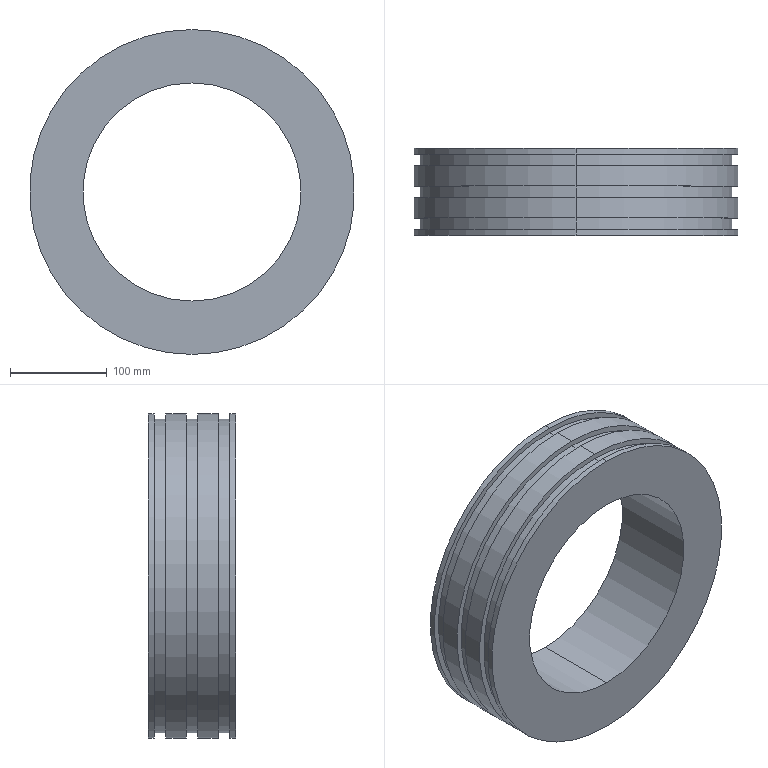Part | SolidWorks | features BaseBody 1, Scale 1 | 1 solid | 24 faces | box 336 x 90 x 336 mm | volume 4158634 mm3 | cylinder 16 | plane 8 | commonest cylinder face diameters 336 x8 324 x6 225.6 x2
STEP:
#1=CARTESIAN_POINT('',(0.,82.5,112.8));
#2=VERTEX_POINT('',#1);
#3=CARTESIAN_POINT('',(0.,82.5,-112.8));
#4=VERTEX_POINT('',#3);
#5=CARTESIAN_POINT('',(0.,82.5,0.));
#6=DIRECTION('',(0.,-1.,0.));
#7=DIRECTION('',(0.,0.,-1.));
#8=AXIS2_PLACEMENT_3D('',#5,#6,#7);
#9=CIRCLE('',#8,112.8);
#10=EDGE_CURVE('',#2,#4,#9,.T.);
#11=ORIENTED_EDGE('',*,*,#10,.F.);
#12=CARTESIAN_POINT('',(0.,-7.5,112.8));
#13=VERTEX_POINT('',#12);
#14=CARTESIAN_POINT('',(0.,82.5,112.8));
#15=DIRECTION('',(0.,-1.,0.));
#16=VECTOR('',#15,1000.);
#17=LINE('',#14,#16);
#18=EDGE_CURVE('',#2,#13,#17,.T.);
#19=ORIENTED_EDGE('',*,*,#18,.T.);
#20=CARTESIAN_POINT('',(0.,-7.5,-112.8));
#21=VERTEX_POINT('',#20);
#22=CARTESIAN_POINT('',(0.,-7.5,0.));
#23=DIRECTION('',(0.,1.,0.));
#24=DIRECTION('',(0.,0.,-1.));
#25=AXIS2_PLACEMENT_3D('',#22,#23,#24);
#26=CIRCLE('',#25,112.8);
#27=EDGE_CURVE('',#21,#13,#26,.T.);
#28=ORIENTED_EDGE('',*,*,#27,.F.);
#29=CARTESIAN_POINT('',(0.,82.5,-112.8));
#30=DIRECTION('',(0.,-1.,0.));
#31=VECTOR('',#30,1000.);
#32=LINE('',#29,#31);
#33=EDGE_CURVE('',#4,#21,#32,.T.);
#34=ORIENTED_EDGE('',*,*,#33,.F.);
#35=EDGE_LOOP('',(#11,#19,#28,#34));
#36=FACE_OUTER_BOUND('',#35,.T.);
#37=CARTESIAN_POINT('',(0.,82.5,0.));
#38=DIRECTION('',(0.,-1.,0.));
#39=DIRECTION('',(0.,0.,-1.));
#40=AXIS2_PLACEMENT_3D('',#37,#38,#39);
#41=CYLINDRICAL_SURFACE('',#40,112.8);
#42=ADVANCED_FACE('',(#36),#41,.F.);
#43=CARTESIAN_POINT('',(0.,82.5,168.));
#44=VERTEX_POINT('',#43);
#45=CARTESIAN_POINT('',(0.,82.5,-168.));
#46=VERTEX_POINT('',#45);
#47=CARTESIAN_POINT('',(0.,82.5,0.));
#48=DIRECTION('',(0.,1.,0.));
#49=DIRECTION('',(0.,0.,-1.));
#50=AXIS2_PLACEMENT_3D('',#47,#48,#49);
#51=CIRCLE('',#50,168.);
#52=EDGE_CURVE('',#44,#46,#51,.T.);
#53=ORIENTED_EDGE('',*,*,#52,.F.);
#54=CARTESIAN_POINT('',(0.,76.5,168.));
#55=VERTEX_POINT('',#54);
#56=CARTESIAN_POINT('',(0.,82.5,168.));
#57=DIRECTION('',(0.,-1.,0.));
#58=VECTOR('',#57,1000.);
#59=LINE('',#56,#58);
#60=EDGE_CURVE('',#44,#55,#59,.T.);
#61=ORIENTED_EDGE('',*,*,#60,.T.);
#62=CARTESIAN_POINT('',(0.,76.5,-168.));
#63=VERTEX_POINT('',#62);
#64=CARTESIAN_POINT('',(0.,76.5,0.));
#65=DIRECTION('',(0.,1.,0.));
#66=DIRECTION('',(0.,0.,-1.));
#67=AXIS2_PLACEMENT_3D('',#64,#65,#66);
#68=CIRCLE('',#67,168.);
#69=EDGE_CURVE('',#55,#63,#68,.T.);
#70=ORIENTED_EDGE('',*,*,#69,.T.);
#71=CARTESIAN_POINT('',(0.,82.5,-168.));
#72=DIRECTION('',(0.,-1.,0.));
#73=VECTOR('',#72,1000.);
#74=LINE('',#71,#73);
#75=EDGE_CURVE('',#46,#63,#74,.T.);
#76=ORIENTED_EDGE('',*,*,#75,.F.);
#77=EDGE_LOOP('',(#53,#61,#70,#76));
#78=FACE_OUTER_BOUND('',#77,.T.);
#79=CARTESIAN_POINT('',(0.,82.5,0.));
#80=DIRECTION('',(0.,-1.,0.));
#81=DIRECTION('',(0.,0.,-1.));
#82=AXIS2_PLACEMENT_3D('',#79,#80,#81);
#83=CYLINDRICAL_SURFACE('',#82,168.);
#84=ADVANCED_FACE('',(#78),#83,.T.);
#85=CARTESIAN_POINT('',(0.,-1.5,-168.));
#86=VERTEX_POINT('',#85);
#87=CARTESIAN_POINT('',(0.,-1.5,168.));
#88=VERTEX_POINT('',#87);
#89=CARTESIAN_POINT('',(0.,-1.5,0.));
#90=DIRECTION('',(0.,-1.,0.));
#91=DIRECTION('',(0.,0.,-1.));
#92=AXIS2_PLACEMENT_3D('',#89,#90,#91);
#93=CIRCLE('',#92,168.);
#94=EDGE_CURVE('',#86,#88,#93,.T.);
#95=ORIENTED_EDGE('',*,*,#94,.T.);
#96=CARTESIAN_POINT('',(0.,-7.5,168.));
#97=VERTEX_POINT('',#96);
#98=CARTESIAN_POINT('',(0.,82.5,168.));
#99=DIRECTION('',(0.,-1.,0.));
#100=VECTOR('',#99,1000.);
#101=LINE('',#98,#100);
#102=EDGE_CURVE('',#88,#97,#101,.T.);
#103=ORIENTED_EDGE('',*,*,#102,.T.);
#104=CARTESIAN_POINT('',(0.,-7.5,-168.));
#105=VERTEX_POINT('',#104);
#106=CARTESIAN_POINT('',(0.,-7.5,0.));
#107=DIRECTION('',(0.,1.,0.));
#108=DIRECTION('',(0.,0.,-1.));
#109=AXIS2_PLACEMENT_3D('',#106,#107,#108);
#110=CIRCLE('',#109,168.);
#111=EDGE_CURVE('',#97,#105,#110,.T.);
#112=ORIENTED_EDGE('',*,*,#111,.T.);
#113=CARTESIAN_POINT('',(0.,82.5,-168.));
#114=DIRECTION('',(0.,-1.,0.));
#115=VECTOR('',#114,1000.);
#116=LINE('',#113,#115);
#117=EDGE_CURVE('',#86,#105,#116,.T.);
#118=ORIENTED_EDGE('',*,*,#117,.F.);
#119=EDGE_LOOP('',(#95,#103,#112,#118));
#120=FACE_OUTER_BOUND('',#119,.T.);
#121=CARTESIAN_POINT('',(0.,82.5,0.));
#122=DIRECTION('',(0.,-1.,0.));
#123=DIRECTION('',(0.,0.,-1.));
#124=AXIS2_PLACEMENT_3D('',#121,#122,#123);
#125=CYLINDRICAL_SURFACE('',#124,168.);
#126=ADVANCED_FACE('',(#120),#125,.T.);
#127=CARTESIAN_POINT('',(0.,76.5,-162.));
#128=VERTEX_POINT('',#127);
#129=CARTESIAN_POINT('',(0.,76.5,162.));
#130=VERTEX_POINT('',#129);
#131=CARTESIAN_POINT('',(0.,76.5,0.));
#132=DIRECTION('',(0.,-1.,0.));
#133=DIRECTION('',(0.,0.,-1.));
#134=AXIS2_PLACEMENT_3D('',#131,#132,#133);
#135=CIRCLE('',#134,162.);
#136=EDGE_CURVE('',#128,#130,#135,.T.);
#137=ORIENTED_EDGE('',*,*,#136,.T.);
#138=CARTESIAN_POINT('',(0.,64.5,162.));
#139=VERTEX_POINT('',#138);
#140=CARTESIAN_POINT('',(0.,-7.5,162.));
#141=DIRECTION('',(0.,-1.,0.));
#142=VECTOR('',#141,1000.);
#143=LINE('',#140,#142);
#144=EDGE_CURVE('',#130,#139,#143,.T.);
#145=ORIENTED_EDGE('',*,*,#144,.T.);
#146=CARTESIAN_POINT('',(0.,64.5,-162.));
#147=VERTEX_POINT('',#146);
#148=CARTESIAN_POINT('',(0.,64.5,0.));
#149=DIRECTION('',(0.,1.,0.));
#150=DIRECTION('',(0.,0.,-1.));
#151=AXIS2_PLACEMENT_3D('',#148,#149,#150);
#152=CIRCLE('',#151,162.);
#153=EDGE_CURVE('',#139,#147,#152,.T.);
#154=ORIENTED_EDGE('',*,*,#153,.T.);
#155=CARTESIAN_POINT('',(0.,-7.5,-162.));
#156=DIRECTION('',(0.,-1.,0.));
#157=VECTOR('',#156,1000.);
#158=LINE('',#155,#157);
#159=EDGE_CURVE('',#128,#147,#158,.T.);
#160=ORIENTED_EDGE('',*,*,#159,.F.);
#161=EDGE_LOOP('',(#137,#145,#154,#160));
#162=FACE_OUTER_BOUND('',#161,.T.);
#163=CARTESIAN_POINT('',(0.,-7.5,0.));
#164=DIRECTION('',(0.,-1.,0.));
#165=DIRECTION('',(0.,0.,-1.));
#166=AXIS2_PLACEMENT_3D('',#163,#164,#165);
#167=CYLINDRICAL_SURFACE('',#166,162.);
#168=ADVANCED_FACE('',(#162),#167,.T.);
#169=CARTESIAN_POINT('',(0.,10.5,-162.));
#170=VERTEX_POINT('',#169);
#171=CARTESIAN_POINT('',(0.,10.5,162.));
#172=VERTEX_POINT('',#171);
#173=CARTESIAN_POINT('',(0.,10.5,0.));
#174=DIRECTION('',(0.,-1.,0.));
#175=DIRECTION('',(0.,0.,-1.));
#176=AXIS2_PLACEMENT_3D('',#173,#174,#175);
#177=CIRCLE('',#176,162.);
#178=EDGE_CURVE('',#170,#172,#177,.T.);
#179=ORIENTED_EDGE('',*,*,#178,.T.);
#180=CARTESIAN_POINT('',(0.,-1.5,162.));
#181=VERTEX_POINT('',#180);
#182=CARTESIAN_POINT('',(0.,-7.5,162.));
#183=DIRECTION('',(0.,-1.,0.));
#184=VECTOR('',#183,1000.);
#185=LINE('',#182,#184);
#186=EDGE_CURVE('',#172,#181,#185,.T.);
#187=ORIENTED_EDGE('',*,*,#186,.T.);
#188=CARTESIAN_POINT('',(0.,-1.5,-162.));
#189=VERTEX_POINT('',#188);
#190=CARTESIAN_POINT('',(0.,-1.5,0.));
#191=DIRECTION('',(0.,1.,0.));
#192=DIRECTION('',(0.,0.,-1.));
#193=AXIS2_PLACEMENT_3D('',#190,#191,#192);
#194=CIRCLE('',#193,162.);
#195=EDGE_CURVE('',#181,#189,#194,.T.);
#196=ORIENTED_EDGE('',*,*,#195,.T.);
#197=CARTESIAN_POINT('',(0.,-7.5,-162.));
#198=DIRECTION('',(0.,-1.,0.));
#199=VECTOR('',#198,1000.);
#200=LINE('',#197,#199);
#201=EDGE_CURVE('',#170,#189,#200,.T.);
#202=ORIENTED_EDGE('',*,*,#201,.F.);
#203=EDGE_LOOP('',(#179,#187,#196,#202));
#204=FACE_OUTER_BOUND('',#203,.T.);
#205=CARTESIAN_POINT('',(0.,-7.5,0.));
#206=DIRECTION('',(0.,-1.,0.));
#207=DIRECTION('',(0.,0.,-1.));
#208=AXIS2_PLACEMENT_3D('',#205,#206,#207);
#209=CYLINDRICAL_SURFACE('',#208,162.);
#210=ADVANCED_FACE('',(#204),#209,.T.);
#211=CARTESIAN_POINT('',(0.,64.5,-168.));
#212=VERTEX_POINT('',#211);
#213=CARTESIAN_POINT('',(0.,64.5,168.));
#214=VERTEX_POINT('',#213);
#215=CARTESIAN_POINT('',(0.,64.5,0.));
#216=DIRECTION('',(0.,-1.,0.));
#217=DIRECTION('',(0.,0.,-1.));
#218=AXIS2_PLACEMENT_3D('',#215,#216,#217);
#219=CIRCLE('',#218,168.);
#220=EDGE_CURVE('',#212,#214,#219,.T.);
#221=ORIENTED_EDGE('',*,*,#220,.T.);
#222=CARTESIAN_POINT('',(0.,43.5,168.));
#223=VERTEX_POINT('',#222);
#224=CARTESIAN_POINT('',(0.,82.5,168.));
#225=DIRECTION('',(0.,-1.,0.));
#226=VECTOR('',#225,1000.);
#227=LINE('',#224,#226);
#228=EDGE_CURVE('',#214,#223,#227,.T.);
#229=ORIENTED_EDGE('',*,*,#228,.T.);
#230=CARTESIAN_POINT('',(0.,43.5,-168.));
#231=VERTEX_POINT('',#230);
#232=CARTESIAN_POINT('',(0.,43.5,0.));
#233=DIRECTION('',(0.,1.,0.));
#234=DIRECTION('',(0.,0.,-1.));
#235=AXIS2_PLACEMENT_3D('',#232,#233,#234);
#236=CIRCLE('',#235,168.);
#237=EDGE_CURVE('',#223,#231,#236,.T.);
#238=ORIENTED_EDGE('',*,*,#237,.T.);
#239=CARTESIAN_POINT('',(0.,82.5,-168.));
#240=DIRECTION('',(0.,-1.,0.));
#241=VECTOR('',#240,1000.);
#242=LINE('',#239,#241);
#243=EDGE_CURVE('',#212,#231,#242,.T.);
#244=ORIENTED_EDGE('',*,*,#243,.F.);
#245=EDGE_LOOP('',(#221,#229,#238,#244));
#246=FACE_OUTER_BOUND('',#245,.T.);
#247=CARTESIAN_POINT('',(0.,82.5,0.));
#248=DIRECTION('',(0.,-1.,0.));
#249=DIRECTION('',(0.,0.,-1.));
#250=AXIS2_PLACEMENT_3D('',#247,#248,#249);
#251=CYLINDRICAL_SURFACE('',#250,168.);
#252=ADVANCED_FACE('',(#246),#251,.T.);
#253=CARTESIAN_POINT('',(0.,31.5,-168.));
#254=VERTEX_POINT('',#253);
#255=CARTESIAN_POINT('',(0.,31.5,168.));
#256=VERTEX_POINT('',#255);
#257=CARTESIAN_POINT('',(0.,31.5,0.));
#258=DIRECTION('',(0.,-1.,0.));
#259=DIRECTION('',(0.,0.,-1.));
#260=AXIS2_PLACEMENT_3D('',#257,#258,#259);
#261=CIRCLE('',#260,168.);
#262=EDGE_CURVE('',#254,#256,#261,.T.);
#263=ORIENTED_EDGE('',*,*,#262,.T.);
#264=CARTESIAN_POINT('',(0.,10.5,168.));
#265=VERTEX_POINT('',#264);
#266=CARTESIAN_POINT('',(0.,82.5,168.));
#267=DIRECTION('',(0.,-1.,0.));
#268=VECTOR('',#267,1000.);
#269=LINE('',#266,#268);
#270=EDGE_CURVE('',#256,#265,#269,.T.);
#271=ORIENTED_EDGE('',*,*,#270,.T.);
#272=CARTESIAN_POINT('',(0.,10.5,-168.));
#273=VERTEX_POINT('',#272);
#274=CARTESIAN_POINT('',(0.,10.5,0.));
#275=DIRECTION('',(0.,1.,0.));
#276=DIRECTION('',(0.,0.,-1.));
#277=AXIS2_PLACEMENT_3D('',#274,#275,#276);
#278=CIRCLE('',#277,168.);
#279=EDGE_CURVE('',#265,#273,#278,.T.);
#280=ORIENTED_EDGE('',*,*,#279,.T.);
#281=CARTESIAN_POINT('',(0.,82.5,-168.));
#282=DIRECTION('',(0.,-1.,0.));
#283=VECTOR('',#282,1000.);
#284=LINE('',#281,#283);
#285=EDGE_CURVE('',#254,#273,#284,.T.);
#286=ORIENTED_EDGE('',*,*,#285,.F.);
#287=EDGE_LOOP('',(#263,#271,#280,#286));
#288=FACE_OUTER_BOUND('',#287,.T.);
#289=CARTESIAN_POINT('',(0.,82.5,0.));
#290=DIRECTION('',(0.,-1.,0.));
#291=DIRECTION('',(0.,0.,-1.));
#292=AXIS2_PLACEMENT_3D('',#289,#290,#291);
#293=CYLINDRICAL_SURFACE('',#292,168.);
#294=ADVANCED_FACE('',(#288),#293,.T.);
#295=CARTESIAN_POINT('',(0.,43.5,-162.));
#296=VERTEX_POINT('',#295);
#297=CARTESIAN_POINT('',(0.,43.5,162.));
#298=VERTEX_POINT('',#297);
#299=CARTESIAN_POINT('',(0.,43.5,0.));
#300=DIRECTION('',(0.,-1.,0.));
#301=DIRECTION('',(0.,0.,-1.));
#302=AXIS2_PLACEMENT_3D('',#299,#300,#301);
#303=CIRCLE('',#302,162.);
#304=EDGE_CURVE('',#296,#298,#303,.T.);
#305=ORIENTED_EDGE('',*,*,#304,.T.);
#306=CARTESIAN_POINT('',(0.,31.5,162.));
#307=VERTEX_POINT('',#306);
#308=CARTESIAN_POINT('',(0.,-7.5,162.));
#309=DIRECTION('',(0.,-1.,0.));
#310=VECTOR('',#309,1000.);
#311=LINE('',#308,#310);
#312=EDGE_CURVE('',#298,#307,#311,.T.);
#313=ORIENTED_EDGE('',*,*,#312,.T.);
#314=CARTESIAN_POINT('',(0.,31.5,-162.));
#315=VERTEX_POINT('',#314);
#316=CARTESIAN_POINT('',(0.,31.5,0.));
#317=DIRECTION('',(0.,1.,0.));
#318=DIRECTION('',(0.,0.,-1.));
#319=AXIS2_PLACEMENT_3D('',#316,#317,#318);
#320=CIRCLE('',#319,162.);
#321=EDGE_CURVE('',#307,#315,#320,.T.);
#322=ORIENTED_EDGE('',*,*,#321,.T.);
#323=CARTESIAN_POINT('',(0.,-7.5,-162.));
#324=DIRECTION('',(0.,-1.,0.));
#325=VECTOR('',#324,1000.);
#326=LINE('',#323,#325);
#327=EDGE_CURVE('',#296,#315,#326,.T.);
#328=ORIENTED_EDGE('',*,*,#327,.F.);
#329=EDGE_LOOP('',(#305,#313,#322,#328));
#330=FACE_OUTER_BOUND('',#329,.T.);
#331=CARTESIAN_POINT('',(0.,-7.5,0.));
#332=DIRECTION('',(0.,-1.,0.));
#333=DIRECTION('',(0.,0.,-1.));
#334=AXIS2_PLACEMENT_3D('',#331,#332,#333);
#335=CYLINDRICAL_SURFACE('',#334,162.);
#336=ADVANCED_FACE('',(#330),#335,.T.);
#337=CARTESIAN_POINT('',(0.,82.5,0.));
#338=DIRECTION('',(0.,-1.,0.));
#339=DIRECTION('',(0.,0.,-1.));
#340=AXIS2_PLACEMENT_3D('',#337,#338,#339);
#341=CIRCLE('',#340,112.8);
#342=EDGE_CURVE('',#4,#2,#341,.T.);
#343=ORIENTED_EDGE('',*,*,#342,.T.);
#344=ORIENTED_EDGE('',*,*,#10,.T.);
#345=EDGE_LOOP('',(#343,#344));
#346=FACE_BOUND('',#345,.T.);
#347=CARTESIAN_POINT('',(0.,82.5,0.));
#348=DIRECTION('',(0.,1.,0.));
#349=DIRECTION('',(0.,0.,-1.));
#350=AXIS2_PLACEMENT_3D('',#347,#348,#349);
#351=CIRCLE('',#350,168.);
#352=EDGE_CURVE('',#46,#44,#351,.T.);
#353=ORIENTED_EDGE('',*,*,#352,.T.);
#354=ORIENTED_EDGE('',*,*,#52,.T.);
#355=EDGE_LOOP('',(#353,#354));
#356=FACE_OUTER_BOUND('',#355,.T.);
#357=CARTESIAN_POINT('',(0.,82.5,0.));
#358=DIRECTION('',(0.,1.,0.));
#359=DIRECTION('',(0.,0.,1.));
#360=AXIS2_PLACEMENT_3D('',#357,#358,#359);
#361=PLANE('',#360);
#362=ADVANCED_FACE('',(#346,#356),#361,.T.);
#363=ORIENTED_EDGE('',*,*,#18,.F.);
#364=ORIENTED_EDGE('',*,*,#342,.F.);
#365=ORIENTED_EDGE('',*,*,#33,.T.);
#366=CARTESIAN_POINT('',(0.,-7.5,0.));
#367=DIRECTION('',(0.,1.,0.));
#368=DIRECTION('',(0.,0.,-1.));
#369=AXIS2_PLACEMENT_3D('',#366,#367,#368);
#370=CIRCLE('',#369,112.8);
#371=EDGE_CURVE('',#13,#21,#370,.T.);
#372=ORIENTED_EDGE('',*,*,#371,.F.);
#373=EDGE_LOOP('',(#363,#364,#365,#372));
#374=FACE_OUTER_BOUND('',#373,.T.);
#375=CARTESIAN_POINT('',(0.,82.5,0.));
#376=DIRECTION('',(0.,-1.,0.));
#377=DIRECTION('',(0.,0.,-1.));
#378=AXIS2_PLACEMENT_3D('',#375,#376,#377);
#379=CYLINDRICAL_SURFACE('',#378,112.8);
#380=ADVANCED_FACE('',(#374),#379,.F.);
#381=ORIENTED_EDGE('',*,*,#60,.F.);
#382=ORIENTED_EDGE('',*,*,#352,.F.);
#383=ORIENTED_EDGE('',*,*,#75,.T.);
#384=CARTESIAN_POINT('',(0.,76.5,0.));
#385=DIRECTION('',(0.,1.,0.));
#386=DIRECTION('',(0.,0.,-1.));
#387=AXIS2_PLACEMENT_3D('',#384,#385,#386);
#388=CIRCLE('',#387,168.);
#389=EDGE_CURVE('',#63,#55,#388,.T.);
#390=ORIENTED_EDGE('',*,*,#389,.T.);
#391=EDGE_LOOP('',(#381,#382,#383,#390));
#392=FACE_OUTER_BOUND('',#391,.T.);
#393=CARTESIAN_POINT('',(0.,82.5,0.));
#394=DIRECTION('',(0.,-1.,0.));
#395=DIRECTION('',(0.,0.,-1.));
#396=AXIS2_PLACEMENT_3D('',#393,#394,#395);
#397=CYLINDRICAL_SURFACE('',#396,168.);
#398=ADVANCED_FACE('',(#392),#397,.T.);
#399=ORIENTED_EDGE('',*,*,#27,.T.);
#400=ORIENTED_EDGE('',*,*,#371,.T.);
#401=EDGE_LOOP('',(#399,#400));
#402=FACE_BOUND('',#401,.T.);
#403=CARTESIAN_POINT('',(0.,-7.5,0.));
#404=DIRECTION('',(0.,1.,0.));
#405=DIRECTION('',(0.,0.,-1.));
#406=AXIS2_PLACEMENT_3D('',#403,#404,#405);
#407=CIRCLE('',#406,168.);
#408=EDGE_CURVE('',#105,#97,#407,.T.);
#409=ORIENTED_EDGE('',*,*,#408,.F.);
#410=ORIENTED_EDGE('',*,*,#111,.F.);
#411=EDGE_LOOP('',(#409,#410));
#412=FACE_OUTER_BOUND('',#411,.T.);
#413=CARTESIAN_POINT('',(0.,-7.5,0.));
#414=DIRECTION('',(0.,1.,0.));
#415=DIRECTION('',(0.,0.,1.));
#416=AXIS2_PLACEMENT_3D('',#413,#414,#415);
#417=PLANE('',#416);
#418=ADVANCED_FACE('',(#402,#412),#417,.F.);
#419=ORIENTED_EDGE('',*,*,#389,.F.);
#420=ORIENTED_EDGE('',*,*,#69,.F.);
#421=EDGE_LOOP('',(#419,#420));
#422=FACE_OUTER_BOUND('',#421,.T.);
#423=ORIENTED_EDGE('',*,*,#136,.F.);
#424=CARTESIAN_POINT('',(0.,76.5,0.));
#425=DIRECTION('',(0.,-1.,0.));
#426=DIRECTION('',(0.,0.,-1.));
#427=AXIS2_PLACEMENT_3D('',#424,#425,#426);
#428=CIRCLE('',#427,162.);
#429=EDGE_CURVE('',#130,#128,#428,.T.);
#430=ORIENTED_EDGE('',*,*,#429,.F.);
#431=EDGE_LOOP('',(#423,#430));
#432=FACE_BOUND('',#431,.T.);
#433=CARTESIAN_POINT('',(168.,76.5,0.));
#434=DIRECTION('',(0.,1.,0.));
#435=DIRECTION('',(0.,0.,1.));
#436=AXIS2_PLACEMENT_3D('',#433,#434,#435);
#437=PLANE('',#436);
#438=ADVANCED_FACE('',(#422,#432),#437,.F.);
#439=ORIENTED_EDGE('',*,*,#102,.F.);
#440=CARTESIAN_POINT('',(0.,-1.5,0.));
#441=DIRECTION('',(0.,-1.,0.));
#442=DIRECTION('',(0.,0.,-1.));
#443=AXIS2_PLACEMENT_3D('',#440,#441,#442);
#444=CIRCLE('',#443,168.);
#445=EDGE_CURVE('',#88,#86,#444,.T.);
#446=ORIENTED_EDGE('',*,*,#445,.T.);
#447=ORIENTED_EDGE('',*,*,#117,.T.);
#448=ORIENTED_EDGE('',*,*,#408,.T.);
#449=EDGE_LOOP('',(#439,#446,#447,#448));
#450=FACE_OUTER_BOUND('',#449,.T.);
#451=CARTESIAN_POINT('',(0.,82.5,0.));
#452=DIRECTION('',(0.,-1.,0.));
#453=DIRECTION('',(0.,0.,-1.));
#454=AXIS2_PLACEMENT_3D('',#451,#452,#453);
#455=CYLINDRICAL_SURFACE('',#454,168.);
#456=ADVANCED_FACE('',(#450),#455,.T.);
#457=ORIENTED_EDGE('',*,*,#144,.F.);
#458=ORIENTED_EDGE('',*,*,#429,.T.);
#459=ORIENTED_EDGE('',*,*,#159,.T.);
#460=CARTESIAN_POINT('',(0.,64.5,0.));
#461=DIRECTION('',(0.,1.,0.));
#462=DIRECTION('',(0.,0.,-1.));
#463=AXIS2_PLACEMENT_3D('',#460,#461,#462);
#464=CIRCLE('',#463,162.);
#465=EDGE_CURVE('',#147,#139,#464,.T.);
#466=ORIENTED_EDGE('',*,*,#465,.T.);
#467=EDGE_LOOP('',(#457,#458,#459,#466));
#468=FACE_OUTER_BOUND('',#467,.T.);
#469=CARTESIAN_POINT('',(0.,-7.5,0.));
#470=DIRECTION('',(0.,-1.,0.));
#471=DIRECTION('',(0.,0.,-1.));
#472=AXIS2_PLACEMENT_3D('',#469,#470,#471);
#473=CYLINDRICAL_SURFACE('',#472,162.);
#474=ADVANCED_FACE('',(#468),#473,.T.);
#475=CARTESIAN_POINT('',(0.,-1.5,0.));
#476=DIRECTION('',(0.,1.,0.));
#477=DIRECTION('',(0.,0.,-1.));
#478=AXIS2_PLACEMENT_3D('',#475,#476,#477);
#479=CIRCLE('',#478,162.);
#480=EDGE_CURVE('',#189,#181,#479,.T.);
#481=ORIENTED_EDGE('',*,*,#480,.F.);
#482=ORIENTED_EDGE('',*,*,#195,.F.);
#483=EDGE_LOOP('',(#481,#482));
#484=FACE_BOUND('',#483,.T.);
#485=ORIENTED_EDGE('',*,*,#94,.F.);
#486=ORIENTED_EDGE('',*,*,#445,.F.);
#487=EDGE_LOOP('',(#485,#486));
#488=FACE_OUTER_BOUND('',#487,.T.);
#489=CARTESIAN_POINT('',(162.,-1.5,0.));
#490=DIRECTION('',(0.,-1.,0.));
#491=DIRECTION('',(0.,0.,-1.));
#492=AXIS2_PLACEMENT_3D('',#489,#490,#491);
#493=PLANE('',#492);
#494=ADVANCED_FACE('',(#484,#488),#493,.F.);
#495=ORIENTED_EDGE('',*,*,#465,.F.);
#496=ORIENTED_EDGE('',*,*,#153,.F.);
#497=EDGE_LOOP('',(#495,#496));
#498=FACE_BOUND('',#497,.T.);
#499=ORIENTED_EDGE('',*,*,#220,.F.);
#500=CARTESIAN_POINT('',(0.,64.5,0.));
#501=DIRECTION('',(0.,-1.,0.));
#502=DIRECTION('',(0.,0.,-1.));
#503=AXIS2_PLACEMENT_3D('',#500,#501,#502);
#504=CIRCLE('',#503,168.);
#505=EDGE_CURVE('',#214,#212,#504,.T.);
#506=ORIENTED_EDGE('',*,*,#505,.F.);
#507=EDGE_LOOP('',(#499,#506));
#508=FACE_OUTER_BOUND('',#507,.T.);
#509=CARTESIAN_POINT('',(162.,64.5,0.));
#510=DIRECTION('',(0.,-1.,0.));
#511=DIRECTION('',(0.,0.,-1.));
#512=AXIS2_PLACEMENT_3D('',#509,#510,#511);
#513=PLANE('',#512);
#514=ADVANCED_FACE('',(#498,#508),#513,.F.);
#515=ORIENTED_EDGE('',*,*,#186,.F.);
#516=CARTESIAN_POINT('',(0.,10.5,0.));
#517=DIRECTION('',(0.,-1.,0.));
#518=DIRECTION('',(0.,0.,-1.));
#519=AXIS2_PLACEMENT_3D('',#516,#517,#518);
#520=CIRCLE('',#519,162.);
#521=EDGE_CURVE('',#172,#170,#520,.T.);
#522=ORIENTED_EDGE('',*,*,#521,.T.);
#523=ORIENTED_EDGE('',*,*,#201,.T.);
#524=ORIENTED_EDGE('',*,*,#480,.T.);
#525=EDGE_LOOP('',(#515,#522,#523,#524));
#526=FACE_OUTER_BOUND('',#525,.T.);
#527=CARTESIAN_POINT('',(0.,-7.5,0.));
#528=DIRECTION('',(0.,-1.,0.));
#529=DIRECTION('',(0.,0.,-1.));
#530=AXIS2_PLACEMENT_3D('',#527,#528,#529);
#531=CYLINDRICAL_SURFACE('',#530,162.);
#532=ADVANCED_FACE('',(#526),#531,.T.);
#533=ORIENTED_EDGE('',*,*,#228,.F.);
#534=ORIENTED_EDGE('',*,*,#505,.T.);
#535=ORIENTED_EDGE('',*,*,#243,.T.);
#536=CARTESIAN_POINT('',(0.,43.5,0.));
#537=DIRECTION('',(0.,1.,0.));
#538=DIRECTION('',(0.,0.,-1.));
#539=AXIS2_PLACEMENT_3D('',#536,#537,#538);
#540=CIRCLE('',#539,168.);
#541=EDGE_CURVE('',#231,#223,#540,.T.);
#542=ORIENTED_EDGE('',*,*,#541,.T.);
#543=EDGE_LOOP('',(#533,#534,#535,#542));
#544=FACE_OUTER_BOUND('',#543,.T.);
#545=CARTESIAN_POINT('',(0.,82.5,0.));
#546=DIRECTION('',(0.,-1.,0.));
#547=DIRECTION('',(0.,0.,-1.));
#548=AXIS2_PLACEMENT_3D('',#545,#546,#547);
#549=CYLINDRICAL_SURFACE('',#548,168.);
#550=ADVANCED_FACE('',(#544),#549,.T.);
#551=CARTESIAN_POINT('',(0.,10.5,0.));
#552=DIRECTION('',(0.,1.,0.));
#553=DIRECTION('',(0.,0.,-1.));
#554=AXIS2_PLACEMENT_3D('',#551,#552,#553);
#555=CIRCLE('',#554,168.);
#556=EDGE_CURVE('',#273,#265,#555,.T.);
#557=ORIENTED_EDGE('',*,*,#556,.F.);
#558=ORIENTED_EDGE('',*,*,#279,.F.);
#559=EDGE_LOOP('',(#557,#558));
#560=FACE_OUTER_BOUND('',#559,.T.);
#561=ORIENTED_EDGE('',*,*,#178,.F.);
#562=ORIENTED_EDGE('',*,*,#521,.F.);
#563=EDGE_LOOP('',(#561,#562));
#564=FACE_BOUND('',#563,.T.);
#565=CARTESIAN_POINT('',(168.,10.5,0.));
#566=DIRECTION('',(0.,1.,0.));
#567=DIRECTION('',(0.,0.,1.));
#568=AXIS2_PLACEMENT_3D('',#565,#566,#567);
#569=PLANE('',#568);
#570=ADVANCED_FACE('',(#560,#564),#569,.F.);
#571=ORIENTED_EDGE('',*,*,#541,.F.);
#572=ORIENTED_EDGE('',*,*,#237,.F.);
#573=EDGE_LOOP('',(#571,#572));
#574=FACE_OUTER_BOUND('',#573,.T.);
#575=ORIENTED_EDGE('',*,*,#304,.F.);
#576=CARTESIAN_POINT('',(0.,43.5,0.));
#577=DIRECTION('',(0.,-1.,0.));
#578=DIRECTION('',(0.,0.,-1.));
#579=AXIS2_PLACEMENT_3D('',#576,#577,#578);
#580=CIRCLE('',#579,162.);
#581=EDGE_CURVE('',#298,#296,#580,.T.);
#582=ORIENTED_EDGE('',*,*,#581,.F.);
#583=EDGE_LOOP('',(#575,#582));
#584=FACE_BOUND('',#583,.T.);
#585=CARTESIAN_POINT('',(168.,43.5,0.));
#586=DIRECTION('',(0.,1.,0.));
#587=DIRECTION('',(0.,0.,1.));
#588=AXIS2_PLACEMENT_3D('',#585,#586,#587);
#589=PLANE('',#588);
#590=ADVANCED_FACE('',(#574,#584),#589,.F.);
#591=ORIENTED_EDGE('',*,*,#270,.F.);
#592=CARTESIAN_POINT('',(0.,31.5,0.));
#593=DIRECTION('',(0.,-1.,0.));
#594=DIRECTION('',(0.,0.,-1.));
#595=AXIS2_PLACEMENT_3D('',#592,#593,#594);
#596=CIRCLE('',#595,168.);
#597=EDGE_CURVE('',#256,#254,#596,.T.);
#598=ORIENTED_EDGE('',*,*,#597,.T.);
#599=ORIENTED_EDGE('',*,*,#285,.T.);
#600=ORIENTED_EDGE('',*,*,#556,.T.);
#601=EDGE_LOOP('',(#591,#598,#599,#600));
#602=FACE_OUTER_BOUND('',#601,.T.);
#603=CARTESIAN_POINT('',(0.,82.5,0.));
#604=DIRECTION('',(0.,-1.,0.));
#605=DIRECTION('',(0.,0.,-1.));
#606=AXIS2_PLACEMENT_3D('',#603,#604,#605);
#607=CYLINDRICAL_SURFACE('',#606,168.);
#608=ADVANCED_FACE('',(#602),#607,.T.);
#609=ORIENTED_EDGE('',*,*,#312,.F.);
#610=ORIENTED_EDGE('',*,*,#581,.T.);
#611=ORIENTED_EDGE('',*,*,#327,.T.);
#612=CARTESIAN_POINT('',(0.,31.5,0.));
#613=DIRECTION('',(0.,1.,0.));
#614=DIRECTION('',(0.,0.,-1.));
#615=AXIS2_PLACEMENT_3D('',#612,#613,#614);
#616=CIRCLE('',#615,162.);
#617=EDGE_CURVE('',#315,#307,#616,.T.);
#618=ORIENTED_EDGE('',*,*,#617,.T.);
#619=EDGE_LOOP('',(#609,#610,#611,#618));
#620=FACE_OUTER_BOUND('',#619,.T.);
#621=CARTESIAN_POINT('',(0.,-7.5,0.));
#622=DIRECTION('',(0.,-1.,0.));
#623=DIRECTION('',(0.,0.,-1.));
#624=AXIS2_PLACEMENT_3D('',#621,#622,#623);
#625=CYLINDRICAL_SURFACE('',#624,162.);
#626=ADVANCED_FACE('',(#620),#625,.T.);
#627=ORIENTED_EDGE('',*,*,#617,.F.);
#628=ORIENTED_EDGE('',*,*,#321,.F.);
#629=EDGE_LOOP('',(#627,#628));
#630=FACE_BOUND('',#629,.T.);
#631=ORIENTED_EDGE('',*,*,#262,.F.);
#632=ORIENTED_EDGE('',*,*,#597,.F.);
#633=EDGE_LOOP('',(#631,#632));
#634=FACE_OUTER_BOUND('',#633,.T.);
#635=CARTESIAN_POINT('',(162.,31.5,0.));
#636=DIRECTION('',(0.,-1.,0.));
#637=DIRECTION('',(0.,0.,-1.));
#638=AXIS2_PLACEMENT_3D('',#635,#636,#637);
#639=PLANE('',#638);
#640=ADVANCED_FACE('',(#630,#634),#639,.F.);
#641=CLOSED_SHELL('',(#42,#84,#126,#168,#210,#252,#294,#336,#362,#380,#398,#418,#438,#456,#474,#494,#514,#532,#550,#570,#590,#608,#626,#640));
#642=MANIFOLD_SOLID_BREP('',#641);
#643=CARTESIAN_POINT('',(0.,0.,0.));
#644=DIRECTION('',(0.,0.,1.));
#645=DIRECTION('',(1.,0.,0.));
#646=AXIS2_PLACEMENT_3D('',#643,#644,#645);
#647=(LENGTH_UNIT()NAMED_UNIT(*)SI_UNIT(.MILLI.,.METRE.));
#648=UNCERTAINTY_MEASURE_WITH_UNIT(LENGTH_MEASURE(0.00001),#647,'','');
#649=(NAMED_UNIT(*)PLANE_ANGLE_UNIT()SI_UNIT($,.RADIAN.));
#650=(NAMED_UNIT(*)SI_UNIT($,.STERADIAN.)SOLID_ANGLE_UNIT());
#651=(GEOMETRIC_REPRESENTATION_CONTEXT(3)GLOBAL_UNCERTAINTY_ASSIGNED_CONTEXT((#648))GLOBAL_UNIT_ASSIGNED_CONTEXT((#647,#649,#650))REPRESENTATION_CONTEXT('',''));
#652=ADVANCED_BREP_SHAPE_REPRESENTATION('',(#642,#646),#651);